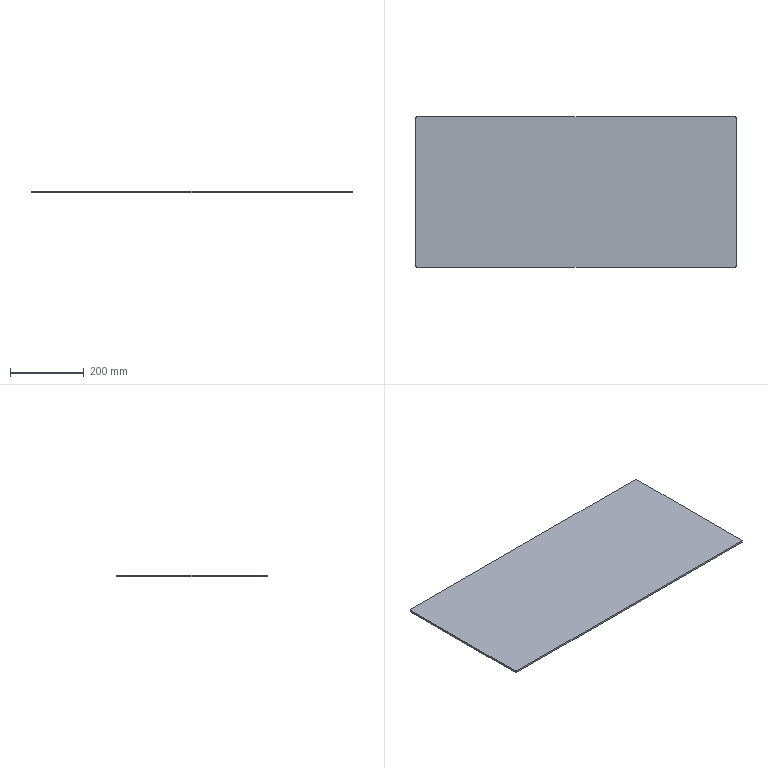Part | STEP file | right front door acrylic cover plate | 1 solid | 10 faces | box 870 x 409 x 5 mm | volume 1779111 mm3 | plane 6 | cylinder 4 | commonest cylinder face diameters 6 x4
STEP:
#1=CARTESIAN_POINT('',(0.,0.,0.));
#2=DIRECTION('',(0.,0.,1.));
#3=DIRECTION('',(1.,0.,0.));
#4=AXIS2_PLACEMENT_3D('',#1,#2,#3);
#5=CARTESIAN_POINT('',(435.,-201.5,5.));
#6=VERTEX_POINT('',#5);
#7=CARTESIAN_POINT('',(435.,201.5,5.));
#8=VERTEX_POINT('',#7);
#9=CARTESIAN_POINT('',(435.,204.5,5.));
#10=DIRECTION('',(0.,1.,0.));
#11=VECTOR('',#10,1.);
#12=LINE('',#9,#11);
#13=CARTESIAN_POINT('',(435.,204.5,5.));
#14=DIRECTION('',(-1.,0.,0.));
#15=DIRECTION('',(0.,-1.,0.));
#16=AXIS2_PLACEMENT_3D('',#13,#14,#15);
#17=PLANE('',#16);
#18=CARTESIAN_POINT('',(0.,0.));
#19=DIRECTION('',(-1.,0.));
#20=VECTOR('',#19,1.);
#21=LINE('',#18,#20);
#22=(GEOMETRIC_REPRESENTATION_CONTEXT(2)PARAMETRIC_REPRESENTATION_CONTEXT()REPRESENTATION_CONTEXT('',''));
#23=DEFINITIONAL_REPRESENTATION('',(#21),#22);
#24=PCURVE('',#17,#23);
#25=CARTESIAN_POINT('',(0.,0.,5.));
#26=DIRECTION('',(0.,0.,1.));
#27=DIRECTION('',(1.,0.,0.));
#28=AXIS2_PLACEMENT_3D('',#25,#26,#27);
#29=PLANE('',#28);
#30=CARTESIAN_POINT('',(435.,204.5));
#31=DIRECTION('',(0.,1.));
#32=VECTOR('',#31,1.);
#33=LINE('',#30,#32);
#34=(GEOMETRIC_REPRESENTATION_CONTEXT(2)PARAMETRIC_REPRESENTATION_CONTEXT()REPRESENTATION_CONTEXT('',''));
#35=DEFINITIONAL_REPRESENTATION('',(#33),#34);
#36=PCURVE('',#29,#35);
#37=SURFACE_CURVE('',#12,(#24,#36),.PCURVE_S1.);
#38=EDGE_CURVE('',#6,#8,#37,.T.);
#39=ORIENTED_EDGE('',*,*,#38,.F.);
#40=CARTESIAN_POINT('',(435.,-201.5,0.));
#41=VERTEX_POINT('',#40);
#42=CARTESIAN_POINT('',(435.,-201.5,5.));
#43=DIRECTION('',(0.,0.,-1.));
#44=VECTOR('',#43,1.);
#45=LINE('',#42,#44);
#46=CARTESIAN_POINT('',(406.,0.));
#47=DIRECTION('',(0.,-1.));
#48=VECTOR('',#47,1.);
#49=LINE('',#46,#48);
#50=(GEOMETRIC_REPRESENTATION_CONTEXT(2)PARAMETRIC_REPRESENTATION_CONTEXT()REPRESENTATION_CONTEXT('',''));
#51=DEFINITIONAL_REPRESENTATION('',(#49),#50);
#52=PCURVE('',#17,#51);
#53=CARTESIAN_POINT('',(432.,-201.5,5.));
#54=DIRECTION('',(0.,0.,-1.));
#55=DIRECTION('',(-1.,0.,0.));
#56=AXIS2_PLACEMENT_3D('',#53,#54,#55);
#57=CYLINDRICAL_SURFACE('',#56,3.);
#58=CARTESIAN_POINT('',(3.142,0.));
#59=DIRECTION('',(0.,1.));
#60=VECTOR('',#59,1.);
#61=LINE('',#58,#60);
#62=(GEOMETRIC_REPRESENTATION_CONTEXT(2)PARAMETRIC_REPRESENTATION_CONTEXT()REPRESENTATION_CONTEXT('',''));
#63=DEFINITIONAL_REPRESENTATION('',(#61),#62);
#64=PCURVE('',#57,#63);
#65=SURFACE_CURVE('',#45,(#52,#64),.PCURVE_S1.);
#66=EDGE_CURVE('',#6,#41,#65,.T.);
#67=ORIENTED_EDGE('',*,*,#66,.T.);
#68=CARTESIAN_POINT('',(435.,201.5,0.));
#69=VERTEX_POINT('',#68);
#70=CARTESIAN_POINT('',(435.,204.5,0.));
#71=DIRECTION('',(0.,1.,0.));
#72=VECTOR('',#71,1.);
#73=LINE('',#70,#72);
#74=CARTESIAN_POINT('',(0.,-5.));
#75=DIRECTION('',(-1.,0.));
#76=VECTOR('',#75,1.);
#77=LINE('',#74,#76);
#78=(GEOMETRIC_REPRESENTATION_CONTEXT(2)PARAMETRIC_REPRESENTATION_CONTEXT()REPRESENTATION_CONTEXT('',''));
#79=DEFINITIONAL_REPRESENTATION('',(#77),#78);
#80=PCURVE('',#17,#79);
#81=CARTESIAN_POINT('',(0.,0.,0.));
#82=DIRECTION('',(0.,0.,1.));
#83=DIRECTION('',(1.,0.,0.));
#84=AXIS2_PLACEMENT_3D('',#81,#82,#83);
#85=PLANE('',#84);
#86=CARTESIAN_POINT('',(435.,204.5));
#87=DIRECTION('',(0.,1.));
#88=VECTOR('',#87,1.);
#89=LINE('',#86,#88);
#90=(GEOMETRIC_REPRESENTATION_CONTEXT(2)PARAMETRIC_REPRESENTATION_CONTEXT()REPRESENTATION_CONTEXT('',''));
#91=DEFINITIONAL_REPRESENTATION('',(#89),#90);
#92=PCURVE('',#85,#91);
#93=SURFACE_CURVE('',#73,(#80,#92),.PCURVE_S1.);
#94=EDGE_CURVE('',#41,#69,#93,.T.);
#95=ORIENTED_EDGE('',*,*,#94,.T.);
#96=CARTESIAN_POINT('',(435.,201.5,5.));
#97=DIRECTION('',(0.,0.,1.));
#98=VECTOR('',#97,1.);
#99=LINE('',#96,#98);
#100=CARTESIAN_POINT('',(3.,0.));
#101=DIRECTION('',(0.,1.));
#102=VECTOR('',#101,1.);
#103=LINE('',#100,#102);
#104=(GEOMETRIC_REPRESENTATION_CONTEXT(2)PARAMETRIC_REPRESENTATION_CONTEXT()REPRESENTATION_CONTEXT('',''));
#105=DEFINITIONAL_REPRESENTATION('',(#103),#104);
#106=PCURVE('',#17,#105);
#107=CARTESIAN_POINT('',(432.,201.5,5.));
#108=DIRECTION('',(0.,0.,-1.));
#109=DIRECTION('',(-1.,0.,0.));
#110=AXIS2_PLACEMENT_3D('',#107,#108,#109);
#111=CYLINDRICAL_SURFACE('',#110,3.);
#112=CARTESIAN_POINT('',(3.142,0.));
#113=DIRECTION('',(0.,-1.));
#114=VECTOR('',#113,1.);
#115=LINE('',#112,#114);
#116=(GEOMETRIC_REPRESENTATION_CONTEXT(2)PARAMETRIC_REPRESENTATION_CONTEXT()REPRESENTATION_CONTEXT('',''));
#117=DEFINITIONAL_REPRESENTATION('',(#115),#116);
#118=PCURVE('',#111,#117);
#119=SURFACE_CURVE('',#99,(#106,#118),.PCURVE_S1.);
#120=EDGE_CURVE('',#69,#8,#119,.T.);
#121=ORIENTED_EDGE('',*,*,#120,.T.);
#122=EDGE_LOOP('',(#39,#67,#95,#121));
#123=FACE_BOUND('',#122,.T.);
#124=ADVANCED_FACE('',(#123),#17,.F.);
#125=CARTESIAN_POINT('',(432.,204.5,0.));
#126=VERTEX_POINT('',#125);
#127=CARTESIAN_POINT('',(-432.,204.5,0.));
#128=VERTEX_POINT('',#127);
#129=CARTESIAN_POINT('',(-435.,204.5,0.));
#130=DIRECTION('',(-1.,0.,0.));
#131=VECTOR('',#130,1.);
#132=LINE('',#129,#131);
#133=CARTESIAN_POINT('',(-435.,204.5,5.));
#134=DIRECTION('',(0.,-1.,0.));
#135=DIRECTION('',(0.,0.,-1.));
#136=AXIS2_PLACEMENT_3D('',#133,#134,#135);
#137=PLANE('',#136);
#138=CARTESIAN_POINT('',(5.,0.));
#139=DIRECTION('',(0.,-1.));
#140=VECTOR('',#139,1.);
#141=LINE('',#138,#140);
#142=(GEOMETRIC_REPRESENTATION_CONTEXT(2)PARAMETRIC_REPRESENTATION_CONTEXT()REPRESENTATION_CONTEXT('',''));
#143=DEFINITIONAL_REPRESENTATION('',(#141),#142);
#144=PCURVE('',#137,#143);
#145=CARTESIAN_POINT('',(-435.,204.5));
#146=DIRECTION('',(-1.,0.));
#147=VECTOR('',#146,1.);
#148=LINE('',#145,#147);
#149=(GEOMETRIC_REPRESENTATION_CONTEXT(2)PARAMETRIC_REPRESENTATION_CONTEXT()REPRESENTATION_CONTEXT('',''));
#150=DEFINITIONAL_REPRESENTATION('',(#148),#149);
#151=PCURVE('',#85,#150);
#152=SURFACE_CURVE('',#132,(#144,#151),.PCURVE_S1.);
#153=EDGE_CURVE('',#126,#128,#152,.T.);
#154=ORIENTED_EDGE('',*,*,#153,.T.);
#155=CARTESIAN_POINT('',(-432.,204.5,5.));
#156=VERTEX_POINT('',#155);
#157=CARTESIAN_POINT('',(-432.,204.5,5.));
#158=DIRECTION('',(0.,0.,1.));
#159=VECTOR('',#158,1.);
#160=LINE('',#157,#159);
#161=CARTESIAN_POINT('',(0.,3.));
#162=DIRECTION('',(-1.,0.));
#163=VECTOR('',#162,1.);
#164=LINE('',#161,#163);
#165=(GEOMETRIC_REPRESENTATION_CONTEXT(2)PARAMETRIC_REPRESENTATION_CONTEXT()REPRESENTATION_CONTEXT('',''));
#166=DEFINITIONAL_REPRESENTATION('',(#164),#165);
#167=PCURVE('',#137,#166);
#168=CARTESIAN_POINT('',(-432.,201.5,5.));
#169=DIRECTION('',(0.,0.,-1.));
#170=DIRECTION('',(-1.,0.,0.));
#171=AXIS2_PLACEMENT_3D('',#168,#169,#170);
#172=CYLINDRICAL_SURFACE('',#171,3.);
#173=CARTESIAN_POINT('',(1.571,0.));
#174=DIRECTION('',(0.,-1.));
#175=VECTOR('',#174,1.);
#176=LINE('',#173,#175);
#177=(GEOMETRIC_REPRESENTATION_CONTEXT(2)PARAMETRIC_REPRESENTATION_CONTEXT()REPRESENTATION_CONTEXT('',''));
#178=DEFINITIONAL_REPRESENTATION('',(#176),#177);
#179=PCURVE('',#172,#178);
#180=SURFACE_CURVE('',#160,(#167,#179),.PCURVE_S1.);
#181=EDGE_CURVE('',#128,#156,#180,.T.);
#182=ORIENTED_EDGE('',*,*,#181,.T.);
#183=CARTESIAN_POINT('',(432.,204.5,5.));
#184=VERTEX_POINT('',#183);
#185=CARTESIAN_POINT('',(-435.,204.5,5.));
#186=DIRECTION('',(-1.,0.,0.));
#187=VECTOR('',#186,1.);
#188=LINE('',#185,#187);
#189=CARTESIAN_POINT('',(0.,0.));
#190=DIRECTION('',(0.,-1.));
#191=VECTOR('',#190,1.);
#192=LINE('',#189,#191);
#193=(GEOMETRIC_REPRESENTATION_CONTEXT(2)PARAMETRIC_REPRESENTATION_CONTEXT()REPRESENTATION_CONTEXT('',''));
#194=DEFINITIONAL_REPRESENTATION('',(#192),#193);
#195=PCURVE('',#137,#194);
#196=CARTESIAN_POINT('',(-435.,204.5));
#197=DIRECTION('',(-1.,0.));
#198=VECTOR('',#197,1.);
#199=LINE('',#196,#198);
#200=(GEOMETRIC_REPRESENTATION_CONTEXT(2)PARAMETRIC_REPRESENTATION_CONTEXT()REPRESENTATION_CONTEXT('',''));
#201=DEFINITIONAL_REPRESENTATION('',(#199),#200);
#202=PCURVE('',#29,#201);
#203=SURFACE_CURVE('',#188,(#195,#202),.PCURVE_S1.);
#204=EDGE_CURVE('',#184,#156,#203,.T.);
#205=ORIENTED_EDGE('',*,*,#204,.F.);
#206=CARTESIAN_POINT('',(432.,204.5,5.));
#207=DIRECTION('',(0.,0.,-1.));
#208=VECTOR('',#207,1.);
#209=LINE('',#206,#208);
#210=CARTESIAN_POINT('',(0.,867.));
#211=DIRECTION('',(1.,0.));
#212=VECTOR('',#211,1.);
#213=LINE('',#210,#212);
#214=(GEOMETRIC_REPRESENTATION_CONTEXT(2)PARAMETRIC_REPRESENTATION_CONTEXT()REPRESENTATION_CONTEXT('',''));
#215=DEFINITIONAL_REPRESENTATION('',(#213),#214);
#216=PCURVE('',#137,#215);
#217=CARTESIAN_POINT('',(1.571,0.));
#218=DIRECTION('',(0.,1.));
#219=VECTOR('',#218,1.);
#220=LINE('',#217,#219);
#221=(GEOMETRIC_REPRESENTATION_CONTEXT(2)PARAMETRIC_REPRESENTATION_CONTEXT()REPRESENTATION_CONTEXT('',''));
#222=DEFINITIONAL_REPRESENTATION('',(#220),#221);
#223=PCURVE('',#111,#222);
#224=SURFACE_CURVE('',#209,(#216,#223),.PCURVE_S1.);
#225=EDGE_CURVE('',#184,#126,#224,.T.);
#226=ORIENTED_EDGE('',*,*,#225,.T.);
#227=EDGE_LOOP('',(#154,#182,#205,#226));
#228=FACE_BOUND('',#227,.T.);
#229=ADVANCED_FACE('',(#228),#137,.F.);
#230=CARTESIAN_POINT('',(-435.,201.5,5.));
#231=VERTEX_POINT('',#230);
#232=CARTESIAN_POINT('',(-435.,-201.5,5.));
#233=VERTEX_POINT('',#232);
#234=CARTESIAN_POINT('',(-435.,204.5,5.));
#235=DIRECTION('',(0.,-1.,0.));
#236=VECTOR('',#235,1.);
#237=LINE('',#234,#236);
#238=CARTESIAN_POINT('',(-435.,204.5,5.));
#239=DIRECTION('',(1.,0.,0.));
#240=DIRECTION('',(0.,1.,0.));
#241=AXIS2_PLACEMENT_3D('',#238,#239,#240);
#242=PLANE('',#241);
#243=CARTESIAN_POINT('',(0.,0.));
#244=DIRECTION('',(-1.,0.));
#245=VECTOR('',#244,1.);
#246=LINE('',#243,#245);
#247=(GEOMETRIC_REPRESENTATION_CONTEXT(2)PARAMETRIC_REPRESENTATION_CONTEXT()REPRESENTATION_CONTEXT('',''));
#248=DEFINITIONAL_REPRESENTATION('',(#246),#247);
#249=PCURVE('',#242,#248);
#250=CARTESIAN_POINT('',(-435.,204.5));
#251=DIRECTION('',(0.,-1.));
#252=VECTOR('',#251,1.);
#253=LINE('',#250,#252);
#254=(GEOMETRIC_REPRESENTATION_CONTEXT(2)PARAMETRIC_REPRESENTATION_CONTEXT()REPRESENTATION_CONTEXT('',''));
#255=DEFINITIONAL_REPRESENTATION('',(#253),#254);
#256=PCURVE('',#29,#255);
#257=SURFACE_CURVE('',#237,(#249,#256),.PCURVE_S1.);
#258=EDGE_CURVE('',#231,#233,#257,.T.);
#259=ORIENTED_EDGE('',*,*,#258,.F.);
#260=CARTESIAN_POINT('',(-435.,201.5,0.));
#261=VERTEX_POINT('',#260);
#262=CARTESIAN_POINT('',(-435.,201.5,5.));
#263=DIRECTION('',(0.,0.,-1.));
#264=VECTOR('',#263,1.);
#265=LINE('',#262,#264);
#266=CARTESIAN_POINT('',(-3.,0.));
#267=DIRECTION('',(0.,-1.));
#268=VECTOR('',#267,1.);
#269=LINE('',#266,#268);
#270=(GEOMETRIC_REPRESENTATION_CONTEXT(2)PARAMETRIC_REPRESENTATION_CONTEXT()REPRESENTATION_CONTEXT('',''));
#271=DEFINITIONAL_REPRESENTATION('',(#269),#270);
#272=PCURVE('',#242,#271);
#273=CARTESIAN_POINT('',(0.,0.));
#274=DIRECTION('',(0.,1.));
#275=VECTOR('',#274,1.);
#276=LINE('',#273,#275);
#277=(GEOMETRIC_REPRESENTATION_CONTEXT(2)PARAMETRIC_REPRESENTATION_CONTEXT()REPRESENTATION_CONTEXT('',''));
#278=DEFINITIONAL_REPRESENTATION('',(#276),#277);
#279=PCURVE('',#172,#278);
#280=SURFACE_CURVE('',#265,(#272,#279),.PCURVE_S1.);
#281=EDGE_CURVE('',#231,#261,#280,.T.);
#282=ORIENTED_EDGE('',*,*,#281,.T.);
#283=CARTESIAN_POINT('',(-435.,-201.5,0.));
#284=VERTEX_POINT('',#283);
#285=CARTESIAN_POINT('',(-435.,204.5,0.));
#286=DIRECTION('',(0.,-1.,0.));
#287=VECTOR('',#286,1.);
#288=LINE('',#285,#287);
#289=CARTESIAN_POINT('',(0.,-5.));
#290=DIRECTION('',(-1.,0.));
#291=VECTOR('',#290,1.);
#292=LINE('',#289,#291);
#293=(GEOMETRIC_REPRESENTATION_CONTEXT(2)PARAMETRIC_REPRESENTATION_CONTEXT()REPRESENTATION_CONTEXT('',''));
#294=DEFINITIONAL_REPRESENTATION('',(#292),#293);
#295=PCURVE('',#242,#294);
#296=CARTESIAN_POINT('',(-435.,204.5));
#297=DIRECTION('',(0.,-1.));
#298=VECTOR('',#297,1.);
#299=LINE('',#296,#298);
#300=(GEOMETRIC_REPRESENTATION_CONTEXT(2)PARAMETRIC_REPRESENTATION_CONTEXT()REPRESENTATION_CONTEXT('',''));
#301=DEFINITIONAL_REPRESENTATION('',(#299),#300);
#302=PCURVE('',#85,#301);
#303=SURFACE_CURVE('',#288,(#295,#302),.PCURVE_S1.);
#304=EDGE_CURVE('',#261,#284,#303,.T.);
#305=ORIENTED_EDGE('',*,*,#304,.T.);
#306=CARTESIAN_POINT('',(-435.,-201.5,5.));
#307=DIRECTION('',(0.,0.,1.));
#308=VECTOR('',#307,1.);
#309=LINE('',#306,#308);
#310=CARTESIAN_POINT('',(-406.,0.));
#311=DIRECTION('',(0.,1.));
#312=VECTOR('',#311,1.);
#313=LINE('',#310,#312);
#314=(GEOMETRIC_REPRESENTATION_CONTEXT(2)PARAMETRIC_REPRESENTATION_CONTEXT()REPRESENTATION_CONTEXT('',''));
#315=DEFINITIONAL_REPRESENTATION('',(#313),#314);
#316=PCURVE('',#242,#315);
#317=CARTESIAN_POINT('',(-432.,-201.5,5.));
#318=DIRECTION('',(0.,0.,-1.));
#319=DIRECTION('',(-1.,0.,0.));
#320=AXIS2_PLACEMENT_3D('',#317,#318,#319);
#321=CYLINDRICAL_SURFACE('',#320,3.);
#322=CARTESIAN_POINT('',(6.283,0.));
#323=DIRECTION('',(0.,-1.));
#324=VECTOR('',#323,1.);
#325=LINE('',#322,#324);
#326=(GEOMETRIC_REPRESENTATION_CONTEXT(2)PARAMETRIC_REPRESENTATION_CONTEXT()REPRESENTATION_CONTEXT('',''));
#327=DEFINITIONAL_REPRESENTATION('',(#325),#326);
#328=PCURVE('',#321,#327);
#329=SURFACE_CURVE('',#309,(#316,#328),.PCURVE_S1.);
#330=EDGE_CURVE('',#284,#233,#329,.T.);
#331=ORIENTED_EDGE('',*,*,#330,.T.);
#332=EDGE_LOOP('',(#259,#282,#305,#331));
#333=FACE_BOUND('',#332,.T.);
#334=ADVANCED_FACE('',(#333),#242,.F.);
#335=CARTESIAN_POINT('',(-432.,-204.5,5.));
#336=VERTEX_POINT('',#335);
#337=CARTESIAN_POINT('',(432.,-204.5,5.));
#338=VERTEX_POINT('',#337);
#339=CARTESIAN_POINT('',(-435.,-204.5,5.));
#340=DIRECTION('',(1.,0.,0.));
#341=VECTOR('',#340,1.);
#342=LINE('',#339,#341);
#343=CARTESIAN_POINT('',(-435.,-204.5,5.));
#344=DIRECTION('',(0.,1.,0.));
#345=DIRECTION('',(0.,0.,1.));
#346=AXIS2_PLACEMENT_3D('',#343,#344,#345);
#347=PLANE('',#346);
#348=CARTESIAN_POINT('',(0.,0.));
#349=DIRECTION('',(0.,1.));
#350=VECTOR('',#349,1.);
#351=LINE('',#348,#350);
#352=(GEOMETRIC_REPRESENTATION_CONTEXT(2)PARAMETRIC_REPRESENTATION_CONTEXT()REPRESENTATION_CONTEXT('',''));
#353=DEFINITIONAL_REPRESENTATION('',(#351),#352);
#354=PCURVE('',#347,#353);
#355=CARTESIAN_POINT('',(-435.,-204.5));
#356=DIRECTION('',(1.,0.));
#357=VECTOR('',#356,1.);
#358=LINE('',#355,#357);
#359=(GEOMETRIC_REPRESENTATION_CONTEXT(2)PARAMETRIC_REPRESENTATION_CONTEXT()REPRESENTATION_CONTEXT('',''));
#360=DEFINITIONAL_REPRESENTATION('',(#358),#359);
#361=PCURVE('',#29,#360);
#362=SURFACE_CURVE('',#342,(#354,#361),.PCURVE_S1.);
#363=EDGE_CURVE('',#336,#338,#362,.T.);
#364=ORIENTED_EDGE('',*,*,#363,.F.);
#365=CARTESIAN_POINT('',(-432.,-204.5,0.));
#366=VERTEX_POINT('',#365);
#367=CARTESIAN_POINT('',(-432.,-204.5,5.));
#368=DIRECTION('',(0.,0.,-1.));
#369=VECTOR('',#368,1.);
#370=LINE('',#367,#369);
#371=CARTESIAN_POINT('',(0.,3.));
#372=DIRECTION('',(-1.,0.));
#373=VECTOR('',#372,1.);
#374=LINE('',#371,#373);
#375=(GEOMETRIC_REPRESENTATION_CONTEXT(2)PARAMETRIC_REPRESENTATION_CONTEXT()REPRESENTATION_CONTEXT('',''));
#376=DEFINITIONAL_REPRESENTATION('',(#374),#375);
#377=PCURVE('',#347,#376);
#378=CARTESIAN_POINT('',(4.712,0.));
#379=DIRECTION('',(0.,1.));
#380=VECTOR('',#379,1.);
#381=LINE('',#378,#380);
#382=(GEOMETRIC_REPRESENTATION_CONTEXT(2)PARAMETRIC_REPRESENTATION_CONTEXT()REPRESENTATION_CONTEXT('',''));
#383=DEFINITIONAL_REPRESENTATION('',(#381),#382);
#384=PCURVE('',#321,#383);
#385=SURFACE_CURVE('',#370,(#377,#384),.PCURVE_S1.);
#386=EDGE_CURVE('',#336,#366,#385,.T.);
#387=ORIENTED_EDGE('',*,*,#386,.T.);
#388=CARTESIAN_POINT('',(432.,-204.5,0.));
#389=VERTEX_POINT('',#388);
#390=CARTESIAN_POINT('',(-435.,-204.5,0.));
#391=DIRECTION('',(1.,0.,0.));
#392=VECTOR('',#391,1.);
#393=LINE('',#390,#392);
#394=CARTESIAN_POINT('',(-5.,0.));
#395=DIRECTION('',(0.,1.));
#396=VECTOR('',#395,1.);
#397=LINE('',#394,#396);
#398=(GEOMETRIC_REPRESENTATION_CONTEXT(2)PARAMETRIC_REPRESENTATION_CONTEXT()REPRESENTATION_CONTEXT('',''));
#399=DEFINITIONAL_REPRESENTATION('',(#397),#398);
#400=PCURVE('',#347,#399);
#401=CARTESIAN_POINT('',(-435.,-204.5));
#402=DIRECTION('',(1.,0.));
#403=VECTOR('',#402,1.);
#404=LINE('',#401,#403);
#405=(GEOMETRIC_REPRESENTATION_CONTEXT(2)PARAMETRIC_REPRESENTATION_CONTEXT()REPRESENTATION_CONTEXT('',''));
#406=DEFINITIONAL_REPRESENTATION('',(#404),#405);
#407=PCURVE('',#85,#406);
#408=SURFACE_CURVE('',#393,(#400,#407),.PCURVE_S1.);
#409=EDGE_CURVE('',#366,#389,#408,.T.);
#410=ORIENTED_EDGE('',*,*,#409,.T.);
#411=CARTESIAN_POINT('',(432.,-204.5,5.));
#412=DIRECTION('',(0.,0.,1.));
#413=VECTOR('',#412,1.);
#414=LINE('',#411,#413);
#415=CARTESIAN_POINT('',(0.,867.));
#416=DIRECTION('',(1.,0.));
#417=VECTOR('',#416,1.);
#418=LINE('',#415,#417);
#419=(GEOMETRIC_REPRESENTATION_CONTEXT(2)PARAMETRIC_REPRESENTATION_CONTEXT()REPRESENTATION_CONTEXT('',''));
#420=DEFINITIONAL_REPRESENTATION('',(#418),#419);
#421=PCURVE('',#347,#420);
#422=CARTESIAN_POINT('',(4.712,0.));
#423=DIRECTION('',(0.,-1.));
#424=VECTOR('',#423,1.);
#425=LINE('',#422,#424);
#426=(GEOMETRIC_REPRESENTATION_CONTEXT(2)PARAMETRIC_REPRESENTATION_CONTEXT()REPRESENTATION_CONTEXT('',''));
#427=DEFINITIONAL_REPRESENTATION('',(#425),#426);
#428=PCURVE('',#57,#427);
#429=SURFACE_CURVE('',#414,(#421,#428),.PCURVE_S1.);
#430=EDGE_CURVE('',#389,#338,#429,.T.);
#431=ORIENTED_EDGE('',*,*,#430,.T.);
#432=EDGE_LOOP('',(#364,#387,#410,#431));
#433=FACE_BOUND('',#432,.T.);
#434=ADVANCED_FACE('',(#433),#347,.F.);
#435=ORIENTED_EDGE('',*,*,#204,.T.);
#436=CARTESIAN_POINT('',(-432.,201.5,5.));
#437=DIRECTION('',(0.,0.,1.));
#438=DIRECTION('',(1.,0.,0.));
#439=AXIS2_PLACEMENT_3D('',#436,#437,#438);
#440=CIRCLE('',#439,3.);
#441=CARTESIAN_POINT('',(-432.,201.5));
#442=DIRECTION('',(1.,0.));
#443=AXIS2_PLACEMENT_2D('',#441,#442);
#444=CIRCLE('',#443,3.);
#445=(GEOMETRIC_REPRESENTATION_CONTEXT(2)PARAMETRIC_REPRESENTATION_CONTEXT()REPRESENTATION_CONTEXT('',''));
#446=DEFINITIONAL_REPRESENTATION('',(#444),#445);
#447=PCURVE('',#29,#446);
#448=CARTESIAN_POINT('',(3.142,0.));
#449=DIRECTION('',(-1.,0.));
#450=VECTOR('',#449,1.);
#451=LINE('',#448,#450);
#452=(GEOMETRIC_REPRESENTATION_CONTEXT(2)PARAMETRIC_REPRESENTATION_CONTEXT()REPRESENTATION_CONTEXT('',''));
#453=DEFINITIONAL_REPRESENTATION('',(#451),#452);
#454=PCURVE('',#172,#453);
#455=SURFACE_CURVE('',#440,(#447,#454),.PCURVE_S1.);
#456=EDGE_CURVE('',#156,#231,#455,.T.);
#457=ORIENTED_EDGE('',*,*,#456,.T.);
#458=ORIENTED_EDGE('',*,*,#258,.T.);
#459=CARTESIAN_POINT('',(-432.,-201.5,5.));
#460=DIRECTION('',(0.,0.,1.));
#461=DIRECTION('',(1.,0.,0.));
#462=AXIS2_PLACEMENT_3D('',#459,#460,#461);
#463=CIRCLE('',#462,3.);
#464=CARTESIAN_POINT('',(-432.,-201.5));
#465=DIRECTION('',(1.,0.));
#466=AXIS2_PLACEMENT_2D('',#464,#465);
#467=CIRCLE('',#466,3.);
#468=(GEOMETRIC_REPRESENTATION_CONTEXT(2)PARAMETRIC_REPRESENTATION_CONTEXT()REPRESENTATION_CONTEXT('',''));
#469=DEFINITIONAL_REPRESENTATION('',(#467),#468);
#470=PCURVE('',#29,#469);
#471=CARTESIAN_POINT('',(9.425,0.));
#472=DIRECTION('',(-1.,0.));
#473=VECTOR('',#472,1.);
#474=LINE('',#471,#473);
#475=(GEOMETRIC_REPRESENTATION_CONTEXT(2)PARAMETRIC_REPRESENTATION_CONTEXT()REPRESENTATION_CONTEXT('',''));
#476=DEFINITIONAL_REPRESENTATION('',(#474),#475);
#477=PCURVE('',#321,#476);
#478=SURFACE_CURVE('',#463,(#470,#477),.PCURVE_S1.);
#479=EDGE_CURVE('',#233,#336,#478,.T.);
#480=ORIENTED_EDGE('',*,*,#479,.T.);
#481=ORIENTED_EDGE('',*,*,#363,.T.);
#482=CARTESIAN_POINT('',(432.,-201.5,5.));
#483=DIRECTION('',(0.,0.,1.));
#484=DIRECTION('',(1.,0.,0.));
#485=AXIS2_PLACEMENT_3D('',#482,#483,#484);
#486=CIRCLE('',#485,3.);
#487=CARTESIAN_POINT('',(432.,-201.5));
#488=DIRECTION('',(1.,0.));
#489=AXIS2_PLACEMENT_2D('',#487,#488);
#490=CIRCLE('',#489,3.);
#491=(GEOMETRIC_REPRESENTATION_CONTEXT(2)PARAMETRIC_REPRESENTATION_CONTEXT()REPRESENTATION_CONTEXT('',''));
#492=DEFINITIONAL_REPRESENTATION('',(#490),#491);
#493=PCURVE('',#29,#492);
#494=CARTESIAN_POINT('',(9.425,0.));
#495=DIRECTION('',(-1.,0.));
#496=VECTOR('',#495,1.);
#497=LINE('',#494,#496);
#498=(GEOMETRIC_REPRESENTATION_CONTEXT(2)PARAMETRIC_REPRESENTATION_CONTEXT()REPRESENTATION_CONTEXT('',''));
#499=DEFINITIONAL_REPRESENTATION('',(#497),#498);
#500=PCURVE('',#57,#499);
#501=SURFACE_CURVE('',#486,(#493,#500),.PCURVE_S1.);
#502=EDGE_CURVE('',#338,#6,#501,.T.);
#503=ORIENTED_EDGE('',*,*,#502,.T.);
#504=ORIENTED_EDGE('',*,*,#38,.T.);
#505=CARTESIAN_POINT('',(432.,201.5,5.));
#506=DIRECTION('',(0.,0.,1.));
#507=DIRECTION('',(1.,0.,0.));
#508=AXIS2_PLACEMENT_3D('',#505,#506,#507);
#509=CIRCLE('',#508,3.);
#510=CARTESIAN_POINT('',(432.,201.5));
#511=DIRECTION('',(1.,0.));
#512=AXIS2_PLACEMENT_2D('',#510,#511);
#513=CIRCLE('',#512,3.);
#514=(GEOMETRIC_REPRESENTATION_CONTEXT(2)PARAMETRIC_REPRESENTATION_CONTEXT()REPRESENTATION_CONTEXT('',''));
#515=DEFINITIONAL_REPRESENTATION('',(#513),#514);
#516=PCURVE('',#29,#515);
#517=CARTESIAN_POINT('',(3.142,0.));
#518=DIRECTION('',(-1.,0.));
#519=VECTOR('',#518,1.);
#520=LINE('',#517,#519);
#521=(GEOMETRIC_REPRESENTATION_CONTEXT(2)PARAMETRIC_REPRESENTATION_CONTEXT()REPRESENTATION_CONTEXT('',''));
#522=DEFINITIONAL_REPRESENTATION('',(#520),#521);
#523=PCURVE('',#111,#522);
#524=SURFACE_CURVE('',#509,(#516,#523),.PCURVE_S1.);
#525=EDGE_CURVE('',#8,#184,#524,.T.);
#526=ORIENTED_EDGE('',*,*,#525,.T.);
#527=EDGE_LOOP('',(#435,#457,#458,#480,#481,#503,#504,#526));
#528=FACE_BOUND('',#527,.T.);
#529=ADVANCED_FACE('',(#528),#29,.T.);
#530=ORIENTED_EDGE('',*,*,#304,.F.);
#531=CARTESIAN_POINT('',(-432.,201.5,0.));
#532=DIRECTION('',(0.,0.,-1.));
#533=DIRECTION('',(1.,0.,0.));
#534=AXIS2_PLACEMENT_3D('',#531,#532,#533);
#535=CIRCLE('',#534,3.);
#536=CARTESIAN_POINT('',(-429.,201.5));
#537=CARTESIAN_POINT('',(-429.,196.304));
#538=CARTESIAN_POINT('',(-433.5,198.902));
#539=CARTESIAN_POINT('',(-438.,201.5));
#540=CARTESIAN_POINT('',(-433.5,204.098));
#541=CARTESIAN_POINT('',(-429.,206.696));
#542=CARTESIAN_POINT('',(-429.,201.5));
#543=(BOUNDED_CURVE()B_SPLINE_CURVE(2,(#536,#537,#538,#539,#540,#541,#542),.UNSPECIFIED.,.T.,.F.)B_SPLINE_CURVE_WITH_KNOTS((1,2,2,2,2,1),(-2.094,0.,2.094,4.189,6.283,8.378),.UNSPECIFIED.)CURVE()GEOMETRIC_REPRESENTATION_ITEM()RATIONAL_B_SPLINE_CURVE((1.,0.5,1.,0.5,1.,0.5,1.))REPRESENTATION_ITEM(''));
#544=(GEOMETRIC_REPRESENTATION_CONTEXT(2)PARAMETRIC_REPRESENTATION_CONTEXT()REPRESENTATION_CONTEXT('',''));
#545=DEFINITIONAL_REPRESENTATION('',(#543),#544);
#546=PCURVE('',#85,#545);
#547=CARTESIAN_POINT('',(-3.142,5.));
#548=DIRECTION('',(1.,0.));
#549=VECTOR('',#548,1.);
#550=LINE('',#547,#549);
#551=(GEOMETRIC_REPRESENTATION_CONTEXT(2)PARAMETRIC_REPRESENTATION_CONTEXT()REPRESENTATION_CONTEXT('',''));
#552=DEFINITIONAL_REPRESENTATION('',(#550),#551);
#553=PCURVE('',#172,#552);
#554=SURFACE_CURVE('',#535,(#546,#553),.PCURVE_S1.);
#555=EDGE_CURVE('',#261,#128,#554,.T.);
#556=ORIENTED_EDGE('',*,*,#555,.T.);
#557=ORIENTED_EDGE('',*,*,#153,.F.);
#558=CARTESIAN_POINT('',(432.,201.5,0.));
#559=DIRECTION('',(0.,0.,-1.));
#560=DIRECTION('',(1.,0.,0.));
#561=AXIS2_PLACEMENT_3D('',#558,#559,#560);
#562=CIRCLE('',#561,3.);
#563=CARTESIAN_POINT('',(435.,201.5));
#564=CARTESIAN_POINT('',(435.,196.304));
#565=CARTESIAN_POINT('',(430.5,198.902));
#566=CARTESIAN_POINT('',(426.,201.5));
#567=CARTESIAN_POINT('',(430.5,204.098));
#568=CARTESIAN_POINT('',(435.,206.696));
#569=CARTESIAN_POINT('',(435.,201.5));
#570=(BOUNDED_CURVE()B_SPLINE_CURVE(2,(#563,#564,#565,#566,#567,#568,#569),.UNSPECIFIED.,.T.,.F.)B_SPLINE_CURVE_WITH_KNOTS((1,2,2,2,2,1),(-2.094,0.,2.094,4.189,6.283,8.378),.UNSPECIFIED.)CURVE()GEOMETRIC_REPRESENTATION_ITEM()RATIONAL_B_SPLINE_CURVE((1.,0.5,1.,0.5,1.,0.5,1.))REPRESENTATION_ITEM(''));
#571=(GEOMETRIC_REPRESENTATION_CONTEXT(2)PARAMETRIC_REPRESENTATION_CONTEXT()REPRESENTATION_CONTEXT('',''));
#572=DEFINITIONAL_REPRESENTATION('',(#570),#571);
#573=PCURVE('',#85,#572);
#574=CARTESIAN_POINT('',(-3.142,5.));
#575=DIRECTION('',(1.,0.));
#576=VECTOR('',#575,1.);
#577=LINE('',#574,#576);
#578=(GEOMETRIC_REPRESENTATION_CONTEXT(2)PARAMETRIC_REPRESENTATION_CONTEXT()REPRESENTATION_CONTEXT('',''));
#579=DEFINITIONAL_REPRESENTATION('',(#577),#578);
#580=PCURVE('',#111,#579);
#581=SURFACE_CURVE('',#562,(#573,#580),.PCURVE_S1.);
#582=EDGE_CURVE('',#126,#69,#581,.T.);
#583=ORIENTED_EDGE('',*,*,#582,.T.);
#584=ORIENTED_EDGE('',*,*,#94,.F.);
#585=CARTESIAN_POINT('',(432.,-201.5,0.));
#586=DIRECTION('',(0.,0.,-1.));
#587=DIRECTION('',(1.,0.,0.));
#588=AXIS2_PLACEMENT_3D('',#585,#586,#587);
#589=CIRCLE('',#588,3.);
#590=CARTESIAN_POINT('',(435.,-201.5));
#591=CARTESIAN_POINT('',(435.,-206.696));
#592=CARTESIAN_POINT('',(430.5,-204.098));
#593=CARTESIAN_POINT('',(426.,-201.5));
#594=CARTESIAN_POINT('',(430.5,-198.902));
#595=CARTESIAN_POINT('',(435.,-196.304));
#596=CARTESIAN_POINT('',(435.,-201.5));
#597=(BOUNDED_CURVE()B_SPLINE_CURVE(2,(#590,#591,#592,#593,#594,#595,#596),.UNSPECIFIED.,.T.,.F.)B_SPLINE_CURVE_WITH_KNOTS((1,2,2,2,2,1),(-2.094,0.,2.094,4.189,6.283,8.378),.UNSPECIFIED.)CURVE()GEOMETRIC_REPRESENTATION_ITEM()RATIONAL_B_SPLINE_CURVE((1.,0.5,1.,0.5,1.,0.5,1.))REPRESENTATION_ITEM(''));
#598=(GEOMETRIC_REPRESENTATION_CONTEXT(2)PARAMETRIC_REPRESENTATION_CONTEXT()REPRESENTATION_CONTEXT('',''));
#599=DEFINITIONAL_REPRESENTATION('',(#597),#598);
#600=PCURVE('',#85,#599);
#601=CARTESIAN_POINT('',(3.142,5.));
#602=DIRECTION('',(1.,0.));
#603=VECTOR('',#602,1.);
#604=LINE('',#601,#603);
#605=(GEOMETRIC_REPRESENTATION_CONTEXT(2)PARAMETRIC_REPRESENTATION_CONTEXT()REPRESENTATION_CONTEXT('',''));
#606=DEFINITIONAL_REPRESENTATION('',(#604),#605);
#607=PCURVE('',#57,#606);
#608=SURFACE_CURVE('',#589,(#600,#607),.PCURVE_S1.);
#609=EDGE_CURVE('',#41,#389,#608,.T.);
#610=ORIENTED_EDGE('',*,*,#609,.T.);
#611=ORIENTED_EDGE('',*,*,#409,.F.);
#612=CARTESIAN_POINT('',(-432.,-201.5,0.));
#613=DIRECTION('',(0.,0.,-1.));
#614=DIRECTION('',(1.,0.,0.));
#615=AXIS2_PLACEMENT_3D('',#612,#613,#614);
#616=CIRCLE('',#615,3.);
#617=CARTESIAN_POINT('',(-429.,-201.5));
#618=CARTESIAN_POINT('',(-429.,-206.696));
#619=CARTESIAN_POINT('',(-433.5,-204.098));
#620=CARTESIAN_POINT('',(-438.,-201.5));
#621=CARTESIAN_POINT('',(-433.5,-198.902));
#622=CARTESIAN_POINT('',(-429.,-196.304));
#623=CARTESIAN_POINT('',(-429.,-201.5));
#624=(BOUNDED_CURVE()B_SPLINE_CURVE(2,(#617,#618,#619,#620,#621,#622,#623),.UNSPECIFIED.,.T.,.F.)B_SPLINE_CURVE_WITH_KNOTS((1,2,2,2,2,1),(-2.094,0.,2.094,4.189,6.283,8.378),.UNSPECIFIED.)CURVE()GEOMETRIC_REPRESENTATION_ITEM()RATIONAL_B_SPLINE_CURVE((1.,0.5,1.,0.5,1.,0.5,1.))REPRESENTATION_ITEM(''));
#625=(GEOMETRIC_REPRESENTATION_CONTEXT(2)PARAMETRIC_REPRESENTATION_CONTEXT()REPRESENTATION_CONTEXT('',''));
#626=DEFINITIONAL_REPRESENTATION('',(#624),#625);
#627=PCURVE('',#85,#626);
#628=CARTESIAN_POINT('',(3.142,5.));
#629=DIRECTION('',(1.,0.));
#630=VECTOR('',#629,1.);
#631=LINE('',#628,#630);
#632=(GEOMETRIC_REPRESENTATION_CONTEXT(2)PARAMETRIC_REPRESENTATION_CONTEXT()REPRESENTATION_CONTEXT('',''));
#633=DEFINITIONAL_REPRESENTATION('',(#631),#632);
#634=PCURVE('',#321,#633);
#635=SURFACE_CURVE('',#616,(#627,#634),.PCURVE_S1.);
#636=EDGE_CURVE('',#366,#284,#635,.T.);
#637=ORIENTED_EDGE('',*,*,#636,.T.);
#638=EDGE_LOOP('',(#530,#556,#557,#583,#584,#610,#611,#637));
#639=FACE_BOUND('',#638,.T.);
#640=ADVANCED_FACE('',(#639),#85,.F.);
#641=ORIENTED_EDGE('',*,*,#456,.F.);
#642=ORIENTED_EDGE('',*,*,#181,.F.);
#643=ORIENTED_EDGE('',*,*,#555,.F.);
#644=ORIENTED_EDGE('',*,*,#281,.F.);
#645=EDGE_LOOP('',(#641,#642,#643,#644));
#646=FACE_BOUND('',#645,.T.);
#647=ADVANCED_FACE('',(#646),#172,.T.);
#648=ORIENTED_EDGE('',*,*,#479,.F.);
#649=ORIENTED_EDGE('',*,*,#330,.F.);
#650=ORIENTED_EDGE('',*,*,#636,.F.);
#651=ORIENTED_EDGE('',*,*,#386,.F.);
#652=EDGE_LOOP('',(#648,#649,#650,#651));
#653=FACE_BOUND('',#652,.T.);
#654=ADVANCED_FACE('',(#653),#321,.T.);
#655=ORIENTED_EDGE('',*,*,#502,.F.);
#656=ORIENTED_EDGE('',*,*,#430,.F.);
#657=ORIENTED_EDGE('',*,*,#609,.F.);
#658=ORIENTED_EDGE('',*,*,#66,.F.);
#659=EDGE_LOOP('',(#655,#656,#657,#658));
#660=FACE_BOUND('',#659,.T.);
#661=ADVANCED_FACE('',(#660),#57,.T.);
#662=ORIENTED_EDGE('',*,*,#525,.F.);
#663=ORIENTED_EDGE('',*,*,#120,.F.);
#664=ORIENTED_EDGE('',*,*,#582,.F.);
#665=ORIENTED_EDGE('',*,*,#225,.F.);
#666=EDGE_LOOP('',(#662,#663,#664,#665));
#667=FACE_BOUND('',#666,.T.);
#668=ADVANCED_FACE('',(#667),#111,.T.);
#669=CLOSED_SHELL('',(#124,#229,#334,#434,#529,#640,#647,#654,#661,#668));
#670=MANIFOLD_SOLID_BREP('',#669);
#671=(LENGTH_UNIT()NAMED_UNIT(*)SI_UNIT(.MILLI.,.METRE.));
#672=UNCERTAINTY_MEASURE_WITH_UNIT(LENGTH_MEASURE(0.0000001),#671,'','');
#673=(NAMED_UNIT(*)PLANE_ANGLE_UNIT()SI_UNIT($,.RADIAN.));
#674=(NAMED_UNIT(*)SI_UNIT($,.STERADIAN.)SOLID_ANGLE_UNIT());
#675=(GEOMETRIC_REPRESENTATION_CONTEXT(3)GLOBAL_UNCERTAINTY_ASSIGNED_CONTEXT((#672))GLOBAL_UNIT_ASSIGNED_CONTEXT((#671,#673,#674))REPRESENTATION_CONTEXT('',''));
#676=ADVANCED_BREP_SHAPE_REPRESENTATION('',(#4,#670),#675);